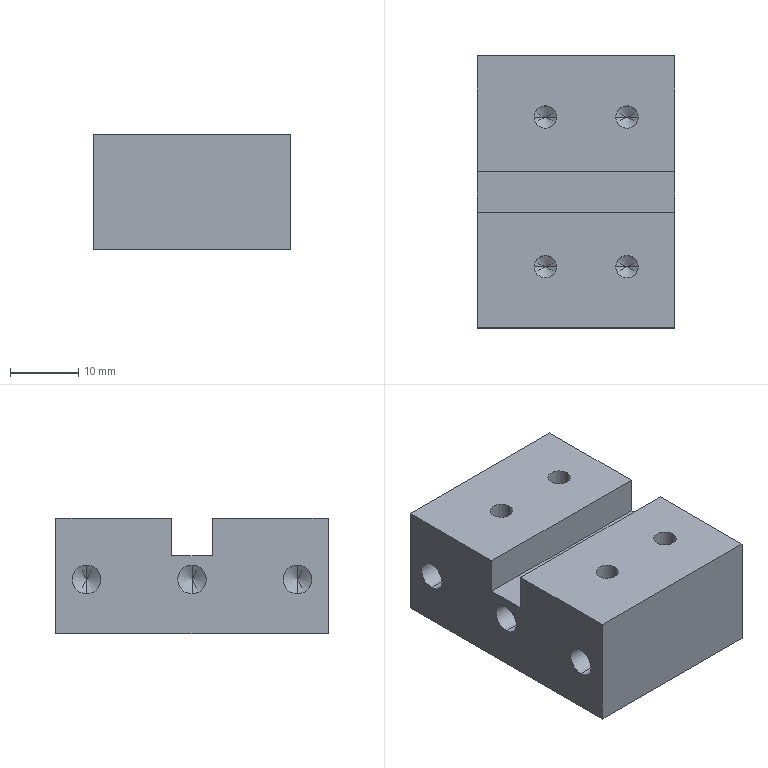Part | NX | features BREP 1 | 1 solid | 38 faces | box 29 x 40 x 17 mm | volume 17873 mm3 | cylinder 14 | cone 14 | plane 10 | commonest cylinder face diameters 3.3 x8 4.2 x6
STEP:
#1=CARTESIAN_POINT('',(-2.6,-15.5,5.9));
#2=VERTEX_POINT('',#1);
#3=CARTESIAN_POINT('',(-2.6,-15.5,10.1));
#4=VERTEX_POINT('',#3);
#5=CARTESIAN_POINT('',(-2.6,-15.5,8.));
#6=DIRECTION('',(-1.,0.,0.));
#7=DIRECTION('',(0.,0.,1.));
#8=AXIS2_PLACEMENT_3D('',#5,#6,#7);
#9=CIRCLE('',#8,2.1);
#10=EDGE_CURVE('',#2,#4,#9,.T.);
#11=ORIENTED_EDGE('',*,*,#10,.F.);
#12=CARTESIAN_POINT('',(-15.,-15.5,5.9));
#13=VERTEX_POINT('',#12);
#14=CARTESIAN_POINT('',(-15.,-15.5,5.9));
#15=DIRECTION('',(-1.,0.,0.));
#16=VECTOR('',#15,1000.);
#17=LINE('',#14,#16);
#18=EDGE_CURVE('',#13,#2,#17,.F.);
#19=ORIENTED_EDGE('',*,*,#18,.F.);
#20=CARTESIAN_POINT('',(-15.,-15.5,10.1));
#21=VERTEX_POINT('',#20);
#22=CARTESIAN_POINT('',(-15.,-15.5,8.));
#23=DIRECTION('',(-1.,0.,0.));
#24=DIRECTION('',(0.,0.,1.));
#25=AXIS2_PLACEMENT_3D('',#22,#23,#24);
#26=CIRCLE('',#25,2.1);
#27=EDGE_CURVE('',#13,#21,#26,.T.);
#28=ORIENTED_EDGE('',*,*,#27,.T.);
#29=CARTESIAN_POINT('',(-15.,-15.5,10.1));
#30=DIRECTION('',(-1.,0.,0.));
#31=VECTOR('',#30,1000.);
#32=LINE('',#29,#31);
#33=EDGE_CURVE('',#21,#4,#32,.F.);
#34=ORIENTED_EDGE('',*,*,#33,.T.);
#35=EDGE_LOOP('',(#11,#19,#28,#34));
#36=FACE_BOUND('',#35,.T.);
#37=CARTESIAN_POINT('',(-15.,-15.5,8.));
#38=DIRECTION('',(-1.,0.,0.));
#39=DIRECTION('',(0.,0.,1.));
#40=AXIS2_PLACEMENT_3D('',#37,#38,#39);
#41=CYLINDRICAL_SURFACE('',#40,2.1);
#42=ADVANCED_FACE('',(#36),#41,.F.);
#43=CARTESIAN_POINT('',(-1.338,-15.5,8.));
#44=VERTEX_POINT('',#43);
#45=CARTESIAN_POINT('',(-2.6,-15.5,10.1));
#46=DIRECTION('',(-0.515,0.,0.8572));
#47=VECTOR('',#46,1000.);
#48=LINE('',#45,#47);
#49=EDGE_CURVE('',#4,#44,#48,.F.);
#50=ORIENTED_EDGE('',*,*,#49,.T.);
#51=CARTESIAN_POINT('',(-2.6,-15.5,5.9));
#52=DIRECTION('',(-0.515,0.,-0.8572));
#53=VECTOR('',#52,1000.);
#54=LINE('',#51,#53);
#55=EDGE_CURVE('',#2,#44,#54,.F.);
#56=ORIENTED_EDGE('',*,*,#55,.F.);
#57=ORIENTED_EDGE('',*,*,#10,.T.);
#58=EDGE_LOOP('',(#50,#56,#57));
#59=FACE_BOUND('',#58,.T.);
#60=CARTESIAN_POINT('',(-2.6,-15.5,8.));
#61=DIRECTION('',(-1.,0.,0.));
#62=DIRECTION('',(0.,0.,1.));
#63=AXIS2_PLACEMENT_3D('',#60,#61,#62);
#64=CONICAL_SURFACE('',#63,2.1,1.03);
#65=ADVANCED_FACE('',(#59),#64,.F.);
#66=CARTESIAN_POINT('',(-2.6,15.5,5.9));
#67=VERTEX_POINT('',#66);
#68=CARTESIAN_POINT('',(-2.6,15.5,10.1));
#69=VERTEX_POINT('',#68);
#70=CARTESIAN_POINT('',(-2.6,15.5,8.));
#71=DIRECTION('',(-1.,0.,0.));
#72=DIRECTION('',(0.,0.,1.));
#73=AXIS2_PLACEMENT_3D('',#70,#71,#72);
#74=CIRCLE('',#73,2.1);
#75=EDGE_CURVE('',#67,#69,#74,.T.);
#76=ORIENTED_EDGE('',*,*,#75,.F.);
#77=CARTESIAN_POINT('',(-15.,15.5,5.9));
#78=VERTEX_POINT('',#77);
#79=CARTESIAN_POINT('',(-15.,15.5,5.9));
#80=DIRECTION('',(-1.,0.,0.));
#81=VECTOR('',#80,1000.);
#82=LINE('',#79,#81);
#83=EDGE_CURVE('',#78,#67,#82,.F.);
#84=ORIENTED_EDGE('',*,*,#83,.F.);
#85=CARTESIAN_POINT('',(-15.,15.5,10.1));
#86=VERTEX_POINT('',#85);
#87=CARTESIAN_POINT('',(-15.,15.5,8.));
#88=DIRECTION('',(-1.,0.,0.));
#89=DIRECTION('',(0.,0.,1.));
#90=AXIS2_PLACEMENT_3D('',#87,#88,#89);
#91=CIRCLE('',#90,2.1);
#92=EDGE_CURVE('',#78,#86,#91,.T.);
#93=ORIENTED_EDGE('',*,*,#92,.T.);
#94=CARTESIAN_POINT('',(-15.,15.5,10.1));
#95=DIRECTION('',(-1.,0.,0.));
#96=VECTOR('',#95,1000.);
#97=LINE('',#94,#96);
#98=EDGE_CURVE('',#86,#69,#97,.F.);
#99=ORIENTED_EDGE('',*,*,#98,.T.);
#100=EDGE_LOOP('',(#76,#84,#93,#99));
#101=FACE_BOUND('',#100,.T.);
#102=CARTESIAN_POINT('',(-15.,15.5,8.));
#103=DIRECTION('',(-1.,0.,0.));
#104=DIRECTION('',(0.,0.,1.));
#105=AXIS2_PLACEMENT_3D('',#102,#103,#104);
#106=CYLINDRICAL_SURFACE('',#105,2.1);
#107=ADVANCED_FACE('',(#101),#106,.F.);
#108=CARTESIAN_POINT('',(-1.338,15.5,8.));
#109=VERTEX_POINT('',#108);
#110=CARTESIAN_POINT('',(-2.6,15.5,10.1));
#111=DIRECTION('',(-0.515,0.,0.8572));
#112=VECTOR('',#111,1000.);
#113=LINE('',#110,#112);
#114=EDGE_CURVE('',#69,#109,#113,.F.);
#115=ORIENTED_EDGE('',*,*,#114,.T.);
#116=CARTESIAN_POINT('',(-2.6,15.5,5.9));
#117=DIRECTION('',(-0.515,0.,-0.8572));
#118=VECTOR('',#117,1000.);
#119=LINE('',#116,#118);
#120=EDGE_CURVE('',#67,#109,#119,.F.);
#121=ORIENTED_EDGE('',*,*,#120,.F.);
#122=ORIENTED_EDGE('',*,*,#75,.T.);
#123=EDGE_LOOP('',(#115,#121,#122));
#124=FACE_BOUND('',#123,.T.);
#125=CARTESIAN_POINT('',(-2.6,15.5,8.));
#126=DIRECTION('',(-1.,0.,0.));
#127=DIRECTION('',(0.,0.,1.));
#128=AXIS2_PLACEMENT_3D('',#125,#126,#127);
#129=CONICAL_SURFACE('',#128,2.1,1.03);
#130=ADVANCED_FACE('',(#124),#129,.F.);
#131=CARTESIAN_POINT('',(-2.6,0.,5.9));
#132=VERTEX_POINT('',#131);
#133=CARTESIAN_POINT('',(-2.6,0.,10.1));
#134=VERTEX_POINT('',#133);
#135=CARTESIAN_POINT('',(-2.6,0.,8.));
#136=DIRECTION('',(-1.,0.,0.));
#137=DIRECTION('',(0.,0.,1.));
#138=AXIS2_PLACEMENT_3D('',#135,#136,#137);
#139=CIRCLE('',#138,2.1);
#140=EDGE_CURVE('',#132,#134,#139,.T.);
#141=ORIENTED_EDGE('',*,*,#140,.F.);
#142=CARTESIAN_POINT('',(-15.,0.,5.9));
#143=VERTEX_POINT('',#142);
#144=CARTESIAN_POINT('',(-15.,0.,5.9));
#145=DIRECTION('',(-1.,0.,0.));
#146=VECTOR('',#145,1000.);
#147=LINE('',#144,#146);
#148=EDGE_CURVE('',#143,#132,#147,.F.);
#149=ORIENTED_EDGE('',*,*,#148,.F.);
#150=CARTESIAN_POINT('',(-15.,0.,10.1));
#151=VERTEX_POINT('',#150);
#152=CARTESIAN_POINT('',(-15.,0.,8.));
#153=DIRECTION('',(-1.,0.,0.));
#154=DIRECTION('',(0.,0.,1.));
#155=AXIS2_PLACEMENT_3D('',#152,#153,#154);
#156=CIRCLE('',#155,2.1);
#157=EDGE_CURVE('',#143,#151,#156,.T.);
#158=ORIENTED_EDGE('',*,*,#157,.T.);
#159=CARTESIAN_POINT('',(-15.,0.,10.1));
#160=DIRECTION('',(-1.,0.,0.));
#161=VECTOR('',#160,1000.);
#162=LINE('',#159,#161);
#163=EDGE_CURVE('',#151,#134,#162,.F.);
#164=ORIENTED_EDGE('',*,*,#163,.T.);
#165=EDGE_LOOP('',(#141,#149,#158,#164));
#166=FACE_BOUND('',#165,.T.);
#167=CARTESIAN_POINT('',(-15.,0.,8.));
#168=DIRECTION('',(-1.,0.,0.));
#169=DIRECTION('',(0.,0.,1.));
#170=AXIS2_PLACEMENT_3D('',#167,#168,#169);
#171=CYLINDRICAL_SURFACE('',#170,2.1);
#172=ADVANCED_FACE('',(#166),#171,.F.);
#173=CARTESIAN_POINT('',(-1.338,0.,8.));
#174=VERTEX_POINT('',#173);
#175=CARTESIAN_POINT('',(-2.6,0.,10.1));
#176=DIRECTION('',(-0.515,0.,0.8572));
#177=VECTOR('',#176,1000.);
#178=LINE('',#175,#177);
#179=EDGE_CURVE('',#134,#174,#178,.F.);
#180=ORIENTED_EDGE('',*,*,#179,.T.);
#181=CARTESIAN_POINT('',(-2.6,0.,5.9));
#182=DIRECTION('',(-0.515,0.,-0.8572));
#183=VECTOR('',#182,1000.);
#184=LINE('',#181,#183);
#185=EDGE_CURVE('',#132,#174,#184,.F.);
#186=ORIENTED_EDGE('',*,*,#185,.F.);
#187=ORIENTED_EDGE('',*,*,#140,.T.);
#188=EDGE_LOOP('',(#180,#186,#187));
#189=FACE_BOUND('',#188,.T.);
#190=CARTESIAN_POINT('',(-2.6,0.,8.));
#191=DIRECTION('',(-1.,0.,0.));
#192=DIRECTION('',(0.,0.,1.));
#193=AXIS2_PLACEMENT_3D('',#190,#191,#192);
#194=CONICAL_SURFACE('',#193,2.1,1.03);
#195=ADVANCED_FACE('',(#189),#194,.F.);
#196=CARTESIAN_POINT('',(-6.65,-11.,6.9));
#197=VERTEX_POINT('',#196);
#198=CARTESIAN_POINT('',(-3.35,-11.,6.9));
#199=VERTEX_POINT('',#198);
#200=CARTESIAN_POINT('',(-5.,-11.,6.9));
#201=DIRECTION('',(0.,0.,1.));
#202=DIRECTION('',(1.,0.,0.));
#203=AXIS2_PLACEMENT_3D('',#200,#201,#202);
#204=CIRCLE('',#203,1.65);
#205=EDGE_CURVE('',#197,#199,#204,.T.);
#206=ORIENTED_EDGE('',*,*,#205,.F.);
#207=CARTESIAN_POINT('',(-6.65,-11.,17.));
#208=VERTEX_POINT('',#207);
#209=CARTESIAN_POINT('',(-6.65,-11.,17.));
#210=DIRECTION('',(0.,0.,1.));
#211=VECTOR('',#210,1000.);
#212=LINE('',#209,#211);
#213=EDGE_CURVE('',#208,#197,#212,.F.);
#214=ORIENTED_EDGE('',*,*,#213,.F.);
#215=CARTESIAN_POINT('',(-3.35,-11.,17.));
#216=VERTEX_POINT('',#215);
#217=CARTESIAN_POINT('',(-5.,-11.,17.));
#218=DIRECTION('',(0.,0.,1.));
#219=DIRECTION('',(1.,0.,0.));
#220=AXIS2_PLACEMENT_3D('',#217,#218,#219);
#221=CIRCLE('',#220,1.65);
#222=EDGE_CURVE('',#208,#216,#221,.T.);
#223=ORIENTED_EDGE('',*,*,#222,.T.);
#224=CARTESIAN_POINT('',(-3.35,-11.,17.));
#225=DIRECTION('',(0.,0.,1.));
#226=VECTOR('',#225,1000.);
#227=LINE('',#224,#226);
#228=EDGE_CURVE('',#216,#199,#227,.F.);
#229=ORIENTED_EDGE('',*,*,#228,.T.);
#230=EDGE_LOOP('',(#206,#214,#223,#229));
#231=FACE_BOUND('',#230,.T.);
#232=CARTESIAN_POINT('',(-5.,-11.,17.));
#233=DIRECTION('',(0.,0.,1.));
#234=DIRECTION('',(1.,0.,0.));
#235=AXIS2_PLACEMENT_3D('',#232,#233,#234);
#236=CYLINDRICAL_SURFACE('',#235,1.65);
#237=ADVANCED_FACE('',(#231),#236,.F.);
#238=CARTESIAN_POINT('',(-5.,-11.,5.909));
#239=VERTEX_POINT('',#238);
#240=CARTESIAN_POINT('',(-3.35,-11.,6.9));
#241=DIRECTION('',(0.8572,0.,0.515));
#242=VECTOR('',#241,1000.);
#243=LINE('',#240,#242);
#244=EDGE_CURVE('',#199,#239,#243,.F.);
#245=ORIENTED_EDGE('',*,*,#244,.T.);
#246=CARTESIAN_POINT('',(-6.65,-11.,6.9));
#247=DIRECTION('',(-0.8572,0.,0.515));
#248=VECTOR('',#247,1000.);
#249=LINE('',#246,#248);
#250=EDGE_CURVE('',#197,#239,#249,.F.);
#251=ORIENTED_EDGE('',*,*,#250,.F.);
#252=ORIENTED_EDGE('',*,*,#205,.T.);
#253=EDGE_LOOP('',(#245,#251,#252));
#254=FACE_BOUND('',#253,.T.);
#255=CARTESIAN_POINT('',(-5.,-11.,6.9));
#256=DIRECTION('',(0.,0.,1.));
#257=DIRECTION('',(1.,0.,0.));
#258=AXIS2_PLACEMENT_3D('',#255,#256,#257);
#259=CONICAL_SURFACE('',#258,1.65,1.03);
#260=ADVANCED_FACE('',(#254),#259,.F.);
#261=CARTESIAN_POINT('',(-6.65,11.,6.9));
#262=VERTEX_POINT('',#261);
#263=CARTESIAN_POINT('',(-3.35,11.,6.9));
#264=VERTEX_POINT('',#263);
#265=CARTESIAN_POINT('',(-5.,11.,6.9));
#266=DIRECTION('',(0.,0.,1.));
#267=DIRECTION('',(1.,0.,0.));
#268=AXIS2_PLACEMENT_3D('',#265,#266,#267);
#269=CIRCLE('',#268,1.65);
#270=EDGE_CURVE('',#262,#264,#269,.T.);
#271=ORIENTED_EDGE('',*,*,#270,.F.);
#272=CARTESIAN_POINT('',(-6.65,11.,17.));
#273=VERTEX_POINT('',#272);
#274=CARTESIAN_POINT('',(-6.65,11.,17.));
#275=DIRECTION('',(0.,0.,1.));
#276=VECTOR('',#275,1000.);
#277=LINE('',#274,#276);
#278=EDGE_CURVE('',#273,#262,#277,.F.);
#279=ORIENTED_EDGE('',*,*,#278,.F.);
#280=CARTESIAN_POINT('',(-3.35,11.,17.));
#281=VERTEX_POINT('',#280);
#282=CARTESIAN_POINT('',(-5.,11.,17.));
#283=DIRECTION('',(0.,0.,1.));
#284=DIRECTION('',(1.,0.,0.));
#285=AXIS2_PLACEMENT_3D('',#282,#283,#284);
#286=CIRCLE('',#285,1.65);
#287=EDGE_CURVE('',#273,#281,#286,.T.);
#288=ORIENTED_EDGE('',*,*,#287,.T.);
#289=CARTESIAN_POINT('',(-3.35,11.,17.));
#290=DIRECTION('',(0.,0.,1.));
#291=VECTOR('',#290,1000.);
#292=LINE('',#289,#291);
#293=EDGE_CURVE('',#281,#264,#292,.F.);
#294=ORIENTED_EDGE('',*,*,#293,.T.);
#295=EDGE_LOOP('',(#271,#279,#288,#294));
#296=FACE_BOUND('',#295,.T.);
#297=CARTESIAN_POINT('',(-5.,11.,17.));
#298=DIRECTION('',(0.,0.,1.));
#299=DIRECTION('',(1.,0.,0.));
#300=AXIS2_PLACEMENT_3D('',#297,#298,#299);
#301=CYLINDRICAL_SURFACE('',#300,1.65);
#302=ADVANCED_FACE('',(#296),#301,.F.);
#303=CARTESIAN_POINT('',(-5.,11.,5.909));
#304=VERTEX_POINT('',#303);
#305=CARTESIAN_POINT('',(-3.35,11.,6.9));
#306=DIRECTION('',(0.8572,0.,0.515));
#307=VECTOR('',#306,1000.);
#308=LINE('',#305,#307);
#309=EDGE_CURVE('',#264,#304,#308,.F.);
#310=ORIENTED_EDGE('',*,*,#309,.T.);
#311=CARTESIAN_POINT('',(-6.65,11.,6.9));
#312=DIRECTION('',(-0.8572,0.,0.515));
#313=VECTOR('',#312,1000.);
#314=LINE('',#311,#313);
#315=EDGE_CURVE('',#262,#304,#314,.F.);
#316=ORIENTED_EDGE('',*,*,#315,.F.);
#317=ORIENTED_EDGE('',*,*,#270,.T.);
#318=EDGE_LOOP('',(#310,#316,#317));
#319=FACE_BOUND('',#318,.T.);
#320=CARTESIAN_POINT('',(-5.,11.,6.9));
#321=DIRECTION('',(0.,0.,1.));
#322=DIRECTION('',(1.,0.,0.));
#323=AXIS2_PLACEMENT_3D('',#320,#321,#322);
#324=CONICAL_SURFACE('',#323,1.65,1.03);
#325=ADVANCED_FACE('',(#319),#324,.F.);
#326=CARTESIAN_POINT('',(5.35,11.,6.9));
#327=VERTEX_POINT('',#326);
#328=CARTESIAN_POINT('',(8.65,11.,6.9));
#329=VERTEX_POINT('',#328);
#330=CARTESIAN_POINT('',(7.,11.,6.9));
#331=DIRECTION('',(0.,0.,1.));
#332=DIRECTION('',(1.,0.,0.));
#333=AXIS2_PLACEMENT_3D('',#330,#331,#332);
#334=CIRCLE('',#333,1.65);
#335=EDGE_CURVE('',#327,#329,#334,.T.);
#336=ORIENTED_EDGE('',*,*,#335,.F.);
#337=CARTESIAN_POINT('',(5.35,11.,17.));
#338=VERTEX_POINT('',#337);
#339=CARTESIAN_POINT('',(5.35,11.,17.));
#340=DIRECTION('',(0.,0.,1.));
#341=VECTOR('',#340,1000.);
#342=LINE('',#339,#341);
#343=EDGE_CURVE('',#338,#327,#342,.F.);
#344=ORIENTED_EDGE('',*,*,#343,.F.);
#345=CARTESIAN_POINT('',(8.65,11.,17.));
#346=VERTEX_POINT('',#345);
#347=CARTESIAN_POINT('',(7.,11.,17.));
#348=DIRECTION('',(0.,0.,1.));
#349=DIRECTION('',(1.,0.,0.));
#350=AXIS2_PLACEMENT_3D('',#347,#348,#349);
#351=CIRCLE('',#350,1.65);
#352=EDGE_CURVE('',#338,#346,#351,.T.);
#353=ORIENTED_EDGE('',*,*,#352,.T.);
#354=CARTESIAN_POINT('',(8.65,11.,17.));
#355=DIRECTION('',(0.,0.,1.));
#356=VECTOR('',#355,1000.);
#357=LINE('',#354,#356);
#358=EDGE_CURVE('',#346,#329,#357,.F.);
#359=ORIENTED_EDGE('',*,*,#358,.T.);
#360=EDGE_LOOP('',(#336,#344,#353,#359));
#361=FACE_BOUND('',#360,.T.);
#362=CARTESIAN_POINT('',(7.,11.,17.));
#363=DIRECTION('',(0.,0.,1.));
#364=DIRECTION('',(1.,0.,0.));
#365=AXIS2_PLACEMENT_3D('',#362,#363,#364);
#366=CYLINDRICAL_SURFACE('',#365,1.65);
#367=ADVANCED_FACE('',(#361),#366,.F.);
#368=CARTESIAN_POINT('',(7.,11.,5.909));
#369=VERTEX_POINT('',#368);
#370=CARTESIAN_POINT('',(8.65,11.,6.9));
#371=DIRECTION('',(0.8572,0.,0.515));
#372=VECTOR('',#371,1000.);
#373=LINE('',#370,#372);
#374=EDGE_CURVE('',#329,#369,#373,.F.);
#375=ORIENTED_EDGE('',*,*,#374,.T.);
#376=CARTESIAN_POINT('',(5.35,11.,6.9));
#377=DIRECTION('',(-0.8572,0.,0.515));
#378=VECTOR('',#377,1000.);
#379=LINE('',#376,#378);
#380=EDGE_CURVE('',#327,#369,#379,.F.);
#381=ORIENTED_EDGE('',*,*,#380,.F.);
#382=ORIENTED_EDGE('',*,*,#335,.T.);
#383=EDGE_LOOP('',(#375,#381,#382));
#384=FACE_BOUND('',#383,.T.);
#385=CARTESIAN_POINT('',(7.,11.,6.9));
#386=DIRECTION('',(0.,0.,1.));
#387=DIRECTION('',(1.,0.,0.));
#388=AXIS2_PLACEMENT_3D('',#385,#386,#387);
#389=CONICAL_SURFACE('',#388,1.65,1.03);
#390=ADVANCED_FACE('',(#384),#389,.F.);
#391=CARTESIAN_POINT('',(5.35,-11.,6.9));
#392=VERTEX_POINT('',#391);
#393=CARTESIAN_POINT('',(8.65,-11.,6.9));
#394=VERTEX_POINT('',#393);
#395=CARTESIAN_POINT('',(7.,-11.,6.9));
#396=DIRECTION('',(0.,0.,1.));
#397=DIRECTION('',(1.,0.,0.));
#398=AXIS2_PLACEMENT_3D('',#395,#396,#397);
#399=CIRCLE('',#398,1.65);
#400=EDGE_CURVE('',#392,#394,#399,.T.);
#401=ORIENTED_EDGE('',*,*,#400,.F.);
#402=CARTESIAN_POINT('',(5.35,-11.,17.));
#403=VERTEX_POINT('',#402);
#404=CARTESIAN_POINT('',(5.35,-11.,17.));
#405=DIRECTION('',(0.,0.,1.));
#406=VECTOR('',#405,1000.);
#407=LINE('',#404,#406);
#408=EDGE_CURVE('',#403,#392,#407,.F.);
#409=ORIENTED_EDGE('',*,*,#408,.F.);
#410=CARTESIAN_POINT('',(8.65,-11.,17.));
#411=VERTEX_POINT('',#410);
#412=CARTESIAN_POINT('',(7.,-11.,17.));
#413=DIRECTION('',(0.,0.,1.));
#414=DIRECTION('',(1.,0.,0.));
#415=AXIS2_PLACEMENT_3D('',#412,#413,#414);
#416=CIRCLE('',#415,1.65);
#417=EDGE_CURVE('',#403,#411,#416,.T.);
#418=ORIENTED_EDGE('',*,*,#417,.T.);
#419=CARTESIAN_POINT('',(8.65,-11.,17.));
#420=DIRECTION('',(0.,0.,1.));
#421=VECTOR('',#420,1000.);
#422=LINE('',#419,#421);
#423=EDGE_CURVE('',#411,#394,#422,.F.);
#424=ORIENTED_EDGE('',*,*,#423,.T.);
#425=EDGE_LOOP('',(#401,#409,#418,#424));
#426=FACE_BOUND('',#425,.T.);
#427=CARTESIAN_POINT('',(7.,-11.,17.));
#428=DIRECTION('',(0.,0.,1.));
#429=DIRECTION('',(1.,0.,0.));
#430=AXIS2_PLACEMENT_3D('',#427,#428,#429);
#431=CYLINDRICAL_SURFACE('',#430,1.65);
#432=ADVANCED_FACE('',(#426),#431,.F.);
#433=CARTESIAN_POINT('',(7.,-11.,5.909));
#434=VERTEX_POINT('',#433);
#435=CARTESIAN_POINT('',(8.65,-11.,6.9));
#436=DIRECTION('',(0.8572,0.,0.515));
#437=VECTOR('',#436,1000.);
#438=LINE('',#435,#437);
#439=EDGE_CURVE('',#394,#434,#438,.F.);
#440=ORIENTED_EDGE('',*,*,#439,.T.);
#441=CARTESIAN_POINT('',(5.35,-11.,6.9));
#442=DIRECTION('',(-0.8572,0.,0.515));
#443=VECTOR('',#442,1000.);
#444=LINE('',#441,#443);
#445=EDGE_CURVE('',#392,#434,#444,.F.);
#446=ORIENTED_EDGE('',*,*,#445,.F.);
#447=ORIENTED_EDGE('',*,*,#400,.T.);
#448=EDGE_LOOP('',(#440,#446,#447));
#449=FACE_BOUND('',#448,.T.);
#450=CARTESIAN_POINT('',(7.,-11.,6.9));
#451=DIRECTION('',(0.,0.,1.));
#452=DIRECTION('',(1.,0.,0.));
#453=AXIS2_PLACEMENT_3D('',#450,#451,#452);
#454=CONICAL_SURFACE('',#453,1.65,1.03);
#455=ADVANCED_FACE('',(#449),#454,.F.);
#456=CARTESIAN_POINT('',(-15.,3.,17.));
#457=VERTEX_POINT('',#456);
#458=CARTESIAN_POINT('',(14.,3.,17.));
#459=VERTEX_POINT('',#458);
#460=CARTESIAN_POINT('',(-15.,3.,17.));
#461=DIRECTION('',(1.,0.,0.));
#462=VECTOR('',#461,1000.);
#463=LINE('',#460,#462);
#464=EDGE_CURVE('',#457,#459,#463,.T.);
#465=ORIENTED_EDGE('',*,*,#464,.T.);
#466=CARTESIAN_POINT('',(14.,20.,17.));
#467=VERTEX_POINT('',#466);
#468=CARTESIAN_POINT('',(14.,20.,17.));
#469=DIRECTION('',(0.,1.,0.));
#470=VECTOR('',#469,1000.);
#471=LINE('',#468,#470);
#472=EDGE_CURVE('',#459,#467,#471,.T.);
#473=ORIENTED_EDGE('',*,*,#472,.T.);
#474=CARTESIAN_POINT('',(-15.,20.,17.));
#475=VERTEX_POINT('',#474);
#476=CARTESIAN_POINT('',(-15.,20.,17.));
#477=DIRECTION('',(-1.,0.,0.));
#478=VECTOR('',#477,1000.);
#479=LINE('',#476,#478);
#480=EDGE_CURVE('',#467,#475,#479,.T.);
#481=ORIENTED_EDGE('',*,*,#480,.T.);
#482=CARTESIAN_POINT('',(-15.,20.,17.));
#483=DIRECTION('',(0.,-1.,0.));
#484=VECTOR('',#483,1000.);
#485=LINE('',#482,#484);
#486=EDGE_CURVE('',#475,#457,#485,.T.);
#487=ORIENTED_EDGE('',*,*,#486,.T.);
#488=EDGE_LOOP('',(#465,#473,#481,#487));
#489=FACE_BOUND('',#488,.T.);
#490=CARTESIAN_POINT('',(-5.,11.,17.));
#491=DIRECTION('',(0.,0.,1.));
#492=DIRECTION('',(1.,0.,0.));
#493=AXIS2_PLACEMENT_3D('',#490,#491,#492);
#494=CIRCLE('',#493,1.65);
#495=EDGE_CURVE('',#281,#273,#494,.T.);
#496=ORIENTED_EDGE('',*,*,#495,.F.);
#497=ORIENTED_EDGE('',*,*,#287,.F.);
#498=EDGE_LOOP('',(#496,#497));
#499=FACE_BOUND('',#498,.T.);
#500=CARTESIAN_POINT('',(7.,11.,17.));
#501=DIRECTION('',(0.,0.,1.));
#502=DIRECTION('',(1.,0.,0.));
#503=AXIS2_PLACEMENT_3D('',#500,#501,#502);
#504=CIRCLE('',#503,1.65);
#505=EDGE_CURVE('',#346,#338,#504,.T.);
#506=ORIENTED_EDGE('',*,*,#505,.F.);
#507=ORIENTED_EDGE('',*,*,#352,.F.);
#508=EDGE_LOOP('',(#506,#507));
#509=FACE_BOUND('',#508,.T.);
#510=CARTESIAN_POINT('',(-15.,-20.,17.));
#511=DIRECTION('',(0.,0.,1.));
#512=DIRECTION('',(1.,0.,0.));
#513=AXIS2_PLACEMENT_3D('',#510,#511,#512);
#514=PLANE('',#513);
#515=ADVANCED_FACE('',(#489,#499,#509),#514,.T.);
#516=CARTESIAN_POINT('',(-15.,-3.,11.5));
#517=VERTEX_POINT('',#516);
#518=CARTESIAN_POINT('',(-15.,3.,11.5));
#519=VERTEX_POINT('',#518);
#520=CARTESIAN_POINT('',(-15.,3.,11.5));
#521=DIRECTION('',(0.,1.,0.));
#522=VECTOR('',#521,1000.);
#523=LINE('',#520,#522);
#524=EDGE_CURVE('',#517,#519,#523,.T.);
#525=ORIENTED_EDGE('',*,*,#524,.T.);
#526=CARTESIAN_POINT('',(-15.,3.,17.));
#527=DIRECTION('',(0.,0.,1.));
#528=VECTOR('',#527,1000.);
#529=LINE('',#526,#528);
#530=EDGE_CURVE('',#519,#457,#529,.T.);
#531=ORIENTED_EDGE('',*,*,#530,.T.);
#532=ORIENTED_EDGE('',*,*,#486,.F.);
#533=CARTESIAN_POINT('',(-15.,20.,0.));
#534=VERTEX_POINT('',#533);
#535=CARTESIAN_POINT('',(-15.,20.,17.));
#536=DIRECTION('',(0.,0.,-1.));
#537=VECTOR('',#536,1000.);
#538=LINE('',#535,#537);
#539=EDGE_CURVE('',#475,#534,#538,.T.);
#540=ORIENTED_EDGE('',*,*,#539,.T.);
#541=CARTESIAN_POINT('',(-15.,-20.,0.));
#542=VERTEX_POINT('',#541);
#543=CARTESIAN_POINT('',(-15.,20.,0.));
#544=DIRECTION('',(0.,-1.,0.));
#545=VECTOR('',#544,1000.);
#546=LINE('',#543,#545);
#547=EDGE_CURVE('',#534,#542,#546,.T.);
#548=ORIENTED_EDGE('',*,*,#547,.T.);
#549=CARTESIAN_POINT('',(-15.,-20.,17.));
#550=VERTEX_POINT('',#549);
#551=CARTESIAN_POINT('',(-15.,-20.,17.));
#552=DIRECTION('',(0.,0.,-1.));
#553=VECTOR('',#552,1000.);
#554=LINE('',#551,#553);
#555=EDGE_CURVE('',#550,#542,#554,.T.);
#556=ORIENTED_EDGE('',*,*,#555,.F.);
#557=CARTESIAN_POINT('',(-15.,-3.,17.));
#558=VERTEX_POINT('',#557);
#559=CARTESIAN_POINT('',(-15.,20.,17.));
#560=DIRECTION('',(0.,-1.,0.));
#561=VECTOR('',#560,1000.);
#562=LINE('',#559,#561);
#563=EDGE_CURVE('',#558,#550,#562,.T.);
#564=ORIENTED_EDGE('',*,*,#563,.F.);
#565=CARTESIAN_POINT('',(-15.,-3.,17.));
#566=DIRECTION('',(0.,0.,-1.));
#567=VECTOR('',#566,1000.);
#568=LINE('',#565,#567);
#569=EDGE_CURVE('',#558,#517,#568,.T.);
#570=ORIENTED_EDGE('',*,*,#569,.T.);
#571=EDGE_LOOP('',(#525,#531,#532,#540,#548,#556,#564,#570));
#572=FACE_BOUND('',#571,.T.);
#573=CARTESIAN_POINT('',(-15.,-15.5,8.));
#574=DIRECTION('',(-1.,0.,0.));
#575=DIRECTION('',(0.,0.,1.));
#576=AXIS2_PLACEMENT_3D('',#573,#574,#575);
#577=CIRCLE('',#576,2.1);
#578=EDGE_CURVE('',#21,#13,#577,.T.);
#579=ORIENTED_EDGE('',*,*,#578,.F.);
#580=ORIENTED_EDGE('',*,*,#27,.F.);
#581=EDGE_LOOP('',(#579,#580));
#582=FACE_BOUND('',#581,.T.);
#583=CARTESIAN_POINT('',(-15.,15.5,8.));
#584=DIRECTION('',(-1.,0.,0.));
#585=DIRECTION('',(0.,0.,1.));
#586=AXIS2_PLACEMENT_3D('',#583,#584,#585);
#587=CIRCLE('',#586,2.1);
#588=EDGE_CURVE('',#86,#78,#587,.T.);
#589=ORIENTED_EDGE('',*,*,#588,.F.);
#590=ORIENTED_EDGE('',*,*,#92,.F.);
#591=EDGE_LOOP('',(#589,#590));
#592=FACE_BOUND('',#591,.T.);
#593=CARTESIAN_POINT('',(-15.,0.,8.));
#594=DIRECTION('',(-1.,0.,0.));
#595=DIRECTION('',(0.,0.,1.));
#596=AXIS2_PLACEMENT_3D('',#593,#594,#595);
#597=CIRCLE('',#596,2.1);
#598=EDGE_CURVE('',#151,#143,#597,.T.);
#599=ORIENTED_EDGE('',*,*,#598,.F.);
#600=ORIENTED_EDGE('',*,*,#157,.F.);
#601=EDGE_LOOP('',(#599,#600));
#602=FACE_BOUND('',#601,.T.);
#603=CARTESIAN_POINT('',(-15.,20.,17.));
#604=DIRECTION('',(1.,0.,0.));
#605=DIRECTION('',(0.,1.,0.));
#606=AXIS2_PLACEMENT_3D('',#603,#604,#605);
#607=PLANE('',#606);
#608=ADVANCED_FACE('',(#572,#582,#592,#602),#607,.F.);
#609=CARTESIAN_POINT('',(14.,-20.,0.));
#610=VERTEX_POINT('',#609);
#611=CARTESIAN_POINT('',(-15.,-20.,0.));
#612=DIRECTION('',(1.,0.,0.));
#613=VECTOR('',#612,1000.);
#614=LINE('',#611,#613);
#615=EDGE_CURVE('',#542,#610,#614,.T.);
#616=ORIENTED_EDGE('',*,*,#615,.T.);
#617=CARTESIAN_POINT('',(14.,-20.,17.));
#618=VERTEX_POINT('',#617);
#619=CARTESIAN_POINT('',(14.,-20.,17.));
#620=DIRECTION('',(0.,0.,-1.));
#621=VECTOR('',#620,1000.);
#622=LINE('',#619,#621);
#623=EDGE_CURVE('',#618,#610,#622,.T.);
#624=ORIENTED_EDGE('',*,*,#623,.F.);
#625=CARTESIAN_POINT('',(-15.,-20.,17.));
#626=DIRECTION('',(1.,0.,0.));
#627=VECTOR('',#626,1000.);
#628=LINE('',#625,#627);
#629=EDGE_CURVE('',#550,#618,#628,.T.);
#630=ORIENTED_EDGE('',*,*,#629,.F.);
#631=ORIENTED_EDGE('',*,*,#555,.T.);
#632=EDGE_LOOP('',(#616,#624,#630,#631));
#633=FACE_BOUND('',#632,.T.);
#634=CARTESIAN_POINT('',(-15.,-20.,17.));
#635=DIRECTION('',(0.,1.,0.));
#636=DIRECTION('',(1.,0.,0.));
#637=AXIS2_PLACEMENT_3D('',#634,#635,#636);
#638=PLANE('',#637);
#639=ADVANCED_FACE('',(#633),#638,.F.);
#640=ORIENTED_EDGE('',*,*,#472,.F.);
#641=CARTESIAN_POINT('',(14.,3.,11.5));
#642=VERTEX_POINT('',#641);
#643=CARTESIAN_POINT('',(14.,3.,17.));
#644=DIRECTION('',(0.,0.,1.));
#645=VECTOR('',#644,1000.);
#646=LINE('',#643,#645);
#647=EDGE_CURVE('',#642,#459,#646,.T.);
#648=ORIENTED_EDGE('',*,*,#647,.F.);
#649=CARTESIAN_POINT('',(14.,-3.,11.5));
#650=VERTEX_POINT('',#649);
#651=CARTESIAN_POINT('',(14.,3.,11.5));
#652=DIRECTION('',(0.,1.,0.));
#653=VECTOR('',#652,1000.);
#654=LINE('',#651,#653);
#655=EDGE_CURVE('',#650,#642,#654,.T.);
#656=ORIENTED_EDGE('',*,*,#655,.F.);
#657=CARTESIAN_POINT('',(14.,-3.,17.));
#658=VERTEX_POINT('',#657);
#659=CARTESIAN_POINT('',(14.,-3.,17.));
#660=DIRECTION('',(0.,0.,-1.));
#661=VECTOR('',#660,1000.);
#662=LINE('',#659,#661);
#663=EDGE_CURVE('',#658,#650,#662,.T.);
#664=ORIENTED_EDGE('',*,*,#663,.F.);
#665=CARTESIAN_POINT('',(14.,20.,17.));
#666=DIRECTION('',(0.,1.,0.));
#667=VECTOR('',#666,1000.);
#668=LINE('',#665,#667);
#669=EDGE_CURVE('',#618,#658,#668,.T.);
#670=ORIENTED_EDGE('',*,*,#669,.F.);
#671=ORIENTED_EDGE('',*,*,#623,.T.);
#672=CARTESIAN_POINT('',(14.,20.,0.));
#673=VERTEX_POINT('',#672);
#674=CARTESIAN_POINT('',(14.,20.,0.));
#675=DIRECTION('',(0.,1.,0.));
#676=VECTOR('',#675,1000.);
#677=LINE('',#674,#676);
#678=EDGE_CURVE('',#610,#673,#677,.T.);
#679=ORIENTED_EDGE('',*,*,#678,.T.);
#680=CARTESIAN_POINT('',(14.,20.,17.));
#681=DIRECTION('',(0.,0.,-1.));
#682=VECTOR('',#681,1000.);
#683=LINE('',#680,#682);
#684=EDGE_CURVE('',#467,#673,#683,.T.);
#685=ORIENTED_EDGE('',*,*,#684,.F.);
#686=EDGE_LOOP('',(#640,#648,#656,#664,#670,#671,#679,#685));
#687=FACE_BOUND('',#686,.T.);
#688=CARTESIAN_POINT('',(14.,20.,17.));
#689=DIRECTION('',(-1.,0.,0.));
#690=DIRECTION('',(0.,1.,0.));
#691=AXIS2_PLACEMENT_3D('',#688,#689,#690);
#692=PLANE('',#691);
#693=ADVANCED_FACE('',(#687),#692,.F.);
#694=CARTESIAN_POINT('',(-15.,20.,0.));
#695=DIRECTION('',(-1.,0.,0.));
#696=VECTOR('',#695,1000.);
#697=LINE('',#694,#696);
#698=EDGE_CURVE('',#673,#534,#697,.T.);
#699=ORIENTED_EDGE('',*,*,#698,.T.);
#700=ORIENTED_EDGE('',*,*,#539,.F.);
#701=ORIENTED_EDGE('',*,*,#480,.F.);
#702=ORIENTED_EDGE('',*,*,#684,.T.);
#703=EDGE_LOOP('',(#699,#700,#701,#702));
#704=FACE_BOUND('',#703,.T.);
#705=CARTESIAN_POINT('',(-15.,20.,17.));
#706=DIRECTION('',(0.,-1.,0.));
#707=DIRECTION('',(0.,0.,-1.));
#708=AXIS2_PLACEMENT_3D('',#705,#706,#707);
#709=PLANE('',#708);
#710=ADVANCED_FACE('',(#704),#709,.F.);
#711=CARTESIAN_POINT('',(-15.,-3.,17.));
#712=DIRECTION('',(1.,0.,0.));
#713=VECTOR('',#712,1000.);
#714=LINE('',#711,#713);
#715=EDGE_CURVE('',#558,#658,#714,.T.);
#716=ORIENTED_EDGE('',*,*,#715,.F.);
#717=ORIENTED_EDGE('',*,*,#563,.T.);
#718=ORIENTED_EDGE('',*,*,#629,.T.);
#719=ORIENTED_EDGE('',*,*,#669,.T.);
#720=EDGE_LOOP('',(#716,#717,#718,#719));
#721=FACE_BOUND('',#720,.T.);
#722=CARTESIAN_POINT('',(-5.,-11.,17.));
#723=DIRECTION('',(0.,0.,1.));
#724=DIRECTION('',(1.,0.,0.));
#725=AXIS2_PLACEMENT_3D('',#722,#723,#724);
#726=CIRCLE('',#725,1.65);
#727=EDGE_CURVE('',#216,#208,#726,.T.);
#728=ORIENTED_EDGE('',*,*,#727,.F.);
#729=ORIENTED_EDGE('',*,*,#222,.F.);
#730=EDGE_LOOP('',(#728,#729));
#731=FACE_BOUND('',#730,.T.);
#732=CARTESIAN_POINT('',(7.,-11.,17.));
#733=DIRECTION('',(0.,0.,1.));
#734=DIRECTION('',(1.,0.,0.));
#735=AXIS2_PLACEMENT_3D('',#732,#733,#734);
#736=CIRCLE('',#735,1.65);
#737=EDGE_CURVE('',#411,#403,#736,.T.);
#738=ORIENTED_EDGE('',*,*,#737,.F.);
#739=ORIENTED_EDGE('',*,*,#417,.F.);
#740=EDGE_LOOP('',(#738,#739));
#741=FACE_BOUND('',#740,.T.);
#742=CARTESIAN_POINT('',(-15.,-20.,17.));
#743=DIRECTION('',(0.,0.,1.));
#744=DIRECTION('',(1.,0.,0.));
#745=AXIS2_PLACEMENT_3D('',#742,#743,#744);
#746=PLANE('',#745);
#747=ADVANCED_FACE('',(#721,#731,#741),#746,.T.);
#748=ORIENTED_EDGE('',*,*,#547,.F.);
#749=ORIENTED_EDGE('',*,*,#698,.F.);
#750=ORIENTED_EDGE('',*,*,#678,.F.);
#751=ORIENTED_EDGE('',*,*,#615,.F.);
#752=EDGE_LOOP('',(#748,#749,#750,#751));
#753=FACE_BOUND('',#752,.T.);
#754=CARTESIAN_POINT('',(-15.,-20.,0.));
#755=DIRECTION('',(0.,0.,1.));
#756=DIRECTION('',(1.,0.,0.));
#757=AXIS2_PLACEMENT_3D('',#754,#755,#756);
#758=PLANE('',#757);
#759=ADVANCED_FACE('',(#753),#758,.F.);
#760=ORIENTED_EDGE('',*,*,#647,.T.);
#761=ORIENTED_EDGE('',*,*,#464,.F.);
#762=ORIENTED_EDGE('',*,*,#530,.F.);
#763=CARTESIAN_POINT('',(-15.,3.,11.5));
#764=DIRECTION('',(1.,0.,0.));
#765=VECTOR('',#764,1000.);
#766=LINE('',#763,#765);
#767=EDGE_CURVE('',#519,#642,#766,.T.);
#768=ORIENTED_EDGE('',*,*,#767,.T.);
#769=EDGE_LOOP('',(#760,#761,#762,#768));
#770=FACE_BOUND('',#769,.T.);
#771=CARTESIAN_POINT('',(-15.,3.,17.));
#772=DIRECTION('',(0.,1.,0.));
#773=DIRECTION('',(0.,0.,-1.));
#774=AXIS2_PLACEMENT_3D('',#771,#772,#773);
#775=PLANE('',#774);
#776=ADVANCED_FACE('',(#770),#775,.F.);
#777=ORIENTED_EDGE('',*,*,#655,.T.);
#778=ORIENTED_EDGE('',*,*,#767,.F.);
#779=ORIENTED_EDGE('',*,*,#524,.F.);
#780=CARTESIAN_POINT('',(-15.,-3.,11.5));
#781=DIRECTION('',(1.,0.,0.));
#782=VECTOR('',#781,1000.);
#783=LINE('',#780,#782);
#784=EDGE_CURVE('',#517,#650,#783,.T.);
#785=ORIENTED_EDGE('',*,*,#784,.T.);
#786=EDGE_LOOP('',(#777,#778,#779,#785));
#787=FACE_BOUND('',#786,.T.);
#788=CARTESIAN_POINT('',(-15.,3.,11.5));
#789=DIRECTION('',(0.,0.,-1.));
#790=DIRECTION('',(0.,-1.,0.));
#791=AXIS2_PLACEMENT_3D('',#788,#789,#790);
#792=PLANE('',#791);
#793=ADVANCED_FACE('',(#787),#792,.F.);
#794=ORIENTED_EDGE('',*,*,#663,.T.);
#795=ORIENTED_EDGE('',*,*,#784,.F.);
#796=ORIENTED_EDGE('',*,*,#569,.F.);
#797=ORIENTED_EDGE('',*,*,#715,.T.);
#798=EDGE_LOOP('',(#794,#795,#796,#797));
#799=FACE_BOUND('',#798,.T.);
#800=CARTESIAN_POINT('',(-15.,-3.,17.));
#801=DIRECTION('',(0.,-1.,0.));
#802=DIRECTION('',(0.,0.,-1.));
#803=AXIS2_PLACEMENT_3D('',#800,#801,#802);
#804=PLANE('',#803);
#805=ADVANCED_FACE('',(#799),#804,.F.);
#806=ORIENTED_EDGE('',*,*,#445,.T.);
#807=ORIENTED_EDGE('',*,*,#439,.F.);
#808=CARTESIAN_POINT('',(7.,-11.,6.9));
#809=DIRECTION('',(0.,0.,1.));
#810=DIRECTION('',(1.,0.,0.));
#811=AXIS2_PLACEMENT_3D('',#808,#809,#810);
#812=CIRCLE('',#811,1.65);
#813=EDGE_CURVE('',#394,#392,#812,.T.);
#814=ORIENTED_EDGE('',*,*,#813,.T.);
#815=EDGE_LOOP('',(#806,#807,#814));
#816=FACE_BOUND('',#815,.T.);
#817=CARTESIAN_POINT('',(7.,-11.,6.9));
#818=DIRECTION('',(0.,0.,1.));
#819=DIRECTION('',(1.,0.,0.));
#820=AXIS2_PLACEMENT_3D('',#817,#818,#819);
#821=CONICAL_SURFACE('',#820,1.65,1.03);
#822=ADVANCED_FACE('',(#816),#821,.F.);
#823=ORIENTED_EDGE('',*,*,#408,.T.);
#824=ORIENTED_EDGE('',*,*,#813,.F.);
#825=ORIENTED_EDGE('',*,*,#423,.F.);
#826=ORIENTED_EDGE('',*,*,#737,.T.);
#827=EDGE_LOOP('',(#823,#824,#825,#826));
#828=FACE_BOUND('',#827,.T.);
#829=CARTESIAN_POINT('',(7.,-11.,17.));
#830=DIRECTION('',(0.,0.,1.));
#831=DIRECTION('',(1.,0.,0.));
#832=AXIS2_PLACEMENT_3D('',#829,#830,#831);
#833=CYLINDRICAL_SURFACE('',#832,1.65);
#834=ADVANCED_FACE('',(#828),#833,.F.);
#835=ORIENTED_EDGE('',*,*,#380,.T.);
#836=ORIENTED_EDGE('',*,*,#374,.F.);
#837=CARTESIAN_POINT('',(7.,11.,6.9));
#838=DIRECTION('',(0.,0.,1.));
#839=DIRECTION('',(1.,0.,0.));
#840=AXIS2_PLACEMENT_3D('',#837,#838,#839);
#841=CIRCLE('',#840,1.65);
#842=EDGE_CURVE('',#329,#327,#841,.T.);
#843=ORIENTED_EDGE('',*,*,#842,.T.);
#844=EDGE_LOOP('',(#835,#836,#843));
#845=FACE_BOUND('',#844,.T.);
#846=CARTESIAN_POINT('',(7.,11.,6.9));
#847=DIRECTION('',(0.,0.,1.));
#848=DIRECTION('',(1.,0.,0.));
#849=AXIS2_PLACEMENT_3D('',#846,#847,#848);
#850=CONICAL_SURFACE('',#849,1.65,1.03);
#851=ADVANCED_FACE('',(#845),#850,.F.);
#852=ORIENTED_EDGE('',*,*,#343,.T.);
#853=ORIENTED_EDGE('',*,*,#842,.F.);
#854=ORIENTED_EDGE('',*,*,#358,.F.);
#855=ORIENTED_EDGE('',*,*,#505,.T.);
#856=EDGE_LOOP('',(#852,#853,#854,#855));
#857=FACE_BOUND('',#856,.T.);
#858=CARTESIAN_POINT('',(7.,11.,17.));
#859=DIRECTION('',(0.,0.,1.));
#860=DIRECTION('',(1.,0.,0.));
#861=AXIS2_PLACEMENT_3D('',#858,#859,#860);
#862=CYLINDRICAL_SURFACE('',#861,1.65);
#863=ADVANCED_FACE('',(#857),#862,.F.);
#864=ORIENTED_EDGE('',*,*,#315,.T.);
#865=ORIENTED_EDGE('',*,*,#309,.F.);
#866=CARTESIAN_POINT('',(-5.,11.,6.9));
#867=DIRECTION('',(0.,0.,1.));
#868=DIRECTION('',(1.,0.,0.));
#869=AXIS2_PLACEMENT_3D('',#866,#867,#868);
#870=CIRCLE('',#869,1.65);
#871=EDGE_CURVE('',#264,#262,#870,.T.);
#872=ORIENTED_EDGE('',*,*,#871,.T.);
#873=EDGE_LOOP('',(#864,#865,#872));
#874=FACE_BOUND('',#873,.T.);
#875=CARTESIAN_POINT('',(-5.,11.,6.9));
#876=DIRECTION('',(0.,0.,1.));
#877=DIRECTION('',(1.,0.,0.));
#878=AXIS2_PLACEMENT_3D('',#875,#876,#877);
#879=CONICAL_SURFACE('',#878,1.65,1.03);
#880=ADVANCED_FACE('',(#874),#879,.F.);
#881=ORIENTED_EDGE('',*,*,#278,.T.);
#882=ORIENTED_EDGE('',*,*,#871,.F.);
#883=ORIENTED_EDGE('',*,*,#293,.F.);
#884=ORIENTED_EDGE('',*,*,#495,.T.);
#885=EDGE_LOOP('',(#881,#882,#883,#884));
#886=FACE_BOUND('',#885,.T.);
#887=CARTESIAN_POINT('',(-5.,11.,17.));
#888=DIRECTION('',(0.,0.,1.));
#889=DIRECTION('',(1.,0.,0.));
#890=AXIS2_PLACEMENT_3D('',#887,#888,#889);
#891=CYLINDRICAL_SURFACE('',#890,1.65);
#892=ADVANCED_FACE('',(#886),#891,.F.);
#893=ORIENTED_EDGE('',*,*,#250,.T.);
#894=ORIENTED_EDGE('',*,*,#244,.F.);
#895=CARTESIAN_POINT('',(-5.,-11.,6.9));
#896=DIRECTION('',(0.,0.,1.));
#897=DIRECTION('',(1.,0.,0.));
#898=AXIS2_PLACEMENT_3D('',#895,#896,#897);
#899=CIRCLE('',#898,1.65);
#900=EDGE_CURVE('',#199,#197,#899,.T.);
#901=ORIENTED_EDGE('',*,*,#900,.T.);
#902=EDGE_LOOP('',(#893,#894,#901));
#903=FACE_BOUND('',#902,.T.);
#904=CARTESIAN_POINT('',(-5.,-11.,6.9));
#905=DIRECTION('',(0.,0.,1.));
#906=DIRECTION('',(1.,0.,0.));
#907=AXIS2_PLACEMENT_3D('',#904,#905,#906);
#908=CONICAL_SURFACE('',#907,1.65,1.03);
#909=ADVANCED_FACE('',(#903),#908,.F.);
#910=ORIENTED_EDGE('',*,*,#213,.T.);
#911=ORIENTED_EDGE('',*,*,#900,.F.);
#912=ORIENTED_EDGE('',*,*,#228,.F.);
#913=ORIENTED_EDGE('',*,*,#727,.T.);
#914=EDGE_LOOP('',(#910,#911,#912,#913));
#915=FACE_BOUND('',#914,.T.);
#916=CARTESIAN_POINT('',(-5.,-11.,17.));
#917=DIRECTION('',(0.,0.,1.));
#918=DIRECTION('',(1.,0.,0.));
#919=AXIS2_PLACEMENT_3D('',#916,#917,#918);
#920=CYLINDRICAL_SURFACE('',#919,1.65);
#921=ADVANCED_FACE('',(#915),#920,.F.);
#922=ORIENTED_EDGE('',*,*,#185,.T.);
#923=ORIENTED_EDGE('',*,*,#179,.F.);
#924=CARTESIAN_POINT('',(-2.6,0.,8.));
#925=DIRECTION('',(-1.,0.,0.));
#926=DIRECTION('',(0.,0.,1.));
#927=AXIS2_PLACEMENT_3D('',#924,#925,#926);
#928=CIRCLE('',#927,2.1);
#929=EDGE_CURVE('',#134,#132,#928,.T.);
#930=ORIENTED_EDGE('',*,*,#929,.T.);
#931=EDGE_LOOP('',(#922,#923,#930));
#932=FACE_BOUND('',#931,.T.);
#933=CARTESIAN_POINT('',(-2.6,0.,8.));
#934=DIRECTION('',(-1.,0.,0.));
#935=DIRECTION('',(0.,0.,1.));
#936=AXIS2_PLACEMENT_3D('',#933,#934,#935);
#937=CONICAL_SURFACE('',#936,2.1,1.03);
#938=ADVANCED_FACE('',(#932),#937,.F.);
#939=ORIENTED_EDGE('',*,*,#148,.T.);
#940=ORIENTED_EDGE('',*,*,#929,.F.);
#941=ORIENTED_EDGE('',*,*,#163,.F.);
#942=ORIENTED_EDGE('',*,*,#598,.T.);
#943=EDGE_LOOP('',(#939,#940,#941,#942));
#944=FACE_BOUND('',#943,.T.);
#945=CARTESIAN_POINT('',(-15.,0.,8.));
#946=DIRECTION('',(-1.,0.,0.));
#947=DIRECTION('',(0.,0.,1.));
#948=AXIS2_PLACEMENT_3D('',#945,#946,#947);
#949=CYLINDRICAL_SURFACE('',#948,2.1);
#950=ADVANCED_FACE('',(#944),#949,.F.);
#951=ORIENTED_EDGE('',*,*,#120,.T.);
#952=ORIENTED_EDGE('',*,*,#114,.F.);
#953=CARTESIAN_POINT('',(-2.6,15.5,8.));
#954=DIRECTION('',(-1.,0.,0.));
#955=DIRECTION('',(0.,0.,1.));
#956=AXIS2_PLACEMENT_3D('',#953,#954,#955);
#957=CIRCLE('',#956,2.1);
#958=EDGE_CURVE('',#69,#67,#957,.T.);
#959=ORIENTED_EDGE('',*,*,#958,.T.);
#960=EDGE_LOOP('',(#951,#952,#959));
#961=FACE_BOUND('',#960,.T.);
#962=CARTESIAN_POINT('',(-2.6,15.5,8.));
#963=DIRECTION('',(-1.,0.,0.));
#964=DIRECTION('',(0.,0.,1.));
#965=AXIS2_PLACEMENT_3D('',#962,#963,#964);
#966=CONICAL_SURFACE('',#965,2.1,1.03);
#967=ADVANCED_FACE('',(#961),#966,.F.);
#968=ORIENTED_EDGE('',*,*,#83,.T.);
#969=ORIENTED_EDGE('',*,*,#958,.F.);
#970=ORIENTED_EDGE('',*,*,#98,.F.);
#971=ORIENTED_EDGE('',*,*,#588,.T.);
#972=EDGE_LOOP('',(#968,#969,#970,#971));
#973=FACE_BOUND('',#972,.T.);
#974=CARTESIAN_POINT('',(-15.,15.5,8.));
#975=DIRECTION('',(-1.,0.,0.));
#976=DIRECTION('',(0.,0.,1.));
#977=AXIS2_PLACEMENT_3D('',#974,#975,#976);
#978=CYLINDRICAL_SURFACE('',#977,2.1);
#979=ADVANCED_FACE('',(#973),#978,.F.);
#980=ORIENTED_EDGE('',*,*,#55,.T.);
#981=ORIENTED_EDGE('',*,*,#49,.F.);
#982=CARTESIAN_POINT('',(-2.6,-15.5,8.));
#983=DIRECTION('',(-1.,0.,0.));
#984=DIRECTION('',(0.,0.,1.));
#985=AXIS2_PLACEMENT_3D('',#982,#983,#984);
#986=CIRCLE('',#985,2.1);
#987=EDGE_CURVE('',#4,#2,#986,.T.);
#988=ORIENTED_EDGE('',*,*,#987,.T.);
#989=EDGE_LOOP('',(#980,#981,#988));
#990=FACE_BOUND('',#989,.T.);
#991=CARTESIAN_POINT('',(-2.6,-15.5,8.));
#992=DIRECTION('',(-1.,0.,0.));
#993=DIRECTION('',(0.,0.,1.));
#994=AXIS2_PLACEMENT_3D('',#991,#992,#993);
#995=CONICAL_SURFACE('',#994,2.1,1.03);
#996=ADVANCED_FACE('',(#990),#995,.F.);
#997=ORIENTED_EDGE('',*,*,#18,.T.);
#998=ORIENTED_EDGE('',*,*,#987,.F.);
#999=ORIENTED_EDGE('',*,*,#33,.F.);
#1000=ORIENTED_EDGE('',*,*,#578,.T.);
#1001=EDGE_LOOP('',(#997,#998,#999,#1000));
#1002=FACE_BOUND('',#1001,.T.);
#1003=CARTESIAN_POINT('',(-15.,-15.5,8.));
#1004=DIRECTION('',(-1.,0.,0.));
#1005=DIRECTION('',(0.,0.,1.));
#1006=AXIS2_PLACEMENT_3D('',#1003,#1004,#1005);
#1007=CYLINDRICAL_SURFACE('',#1006,2.1);
#1008=ADVANCED_FACE('',(#1002),#1007,.F.);
#1009=CLOSED_SHELL('',(#42,#65,#107,#130,#172,#195,#237,#260,#302,#325,#367,#390,#432,#455,#515,#608,#639,#693,#710,#747,#759,#776,#793,#805,#822,#834,#851,#863,#880,#892,#909,#921,#938,#950,#967,#979,#996,#1008));
#1010=MANIFOLD_SOLID_BREP('',#1009);
#1011=(LENGTH_UNIT()NAMED_UNIT(*)SI_UNIT(.MILLI.,.METRE.));
#1012=UNCERTAINTY_MEASURE_WITH_UNIT(LENGTH_MEASURE(0.00001),#1011,'','');
#1013=(NAMED_UNIT(*)PLANE_ANGLE_UNIT()SI_UNIT($,.RADIAN.));
#1014=(NAMED_UNIT(*)SI_UNIT($,.STERADIAN.)SOLID_ANGLE_UNIT());
#1015=(GEOMETRIC_REPRESENTATION_CONTEXT(3)GLOBAL_UNCERTAINTY_ASSIGNED_CONTEXT((#1012))GLOBAL_UNIT_ASSIGNED_CONTEXT((#1011,#1013,#1014))REPRESENTATION_CONTEXT('',''));
#1016=ADVANCED_BREP_SHAPE_REPRESENTATION('',(#1010),#1015);